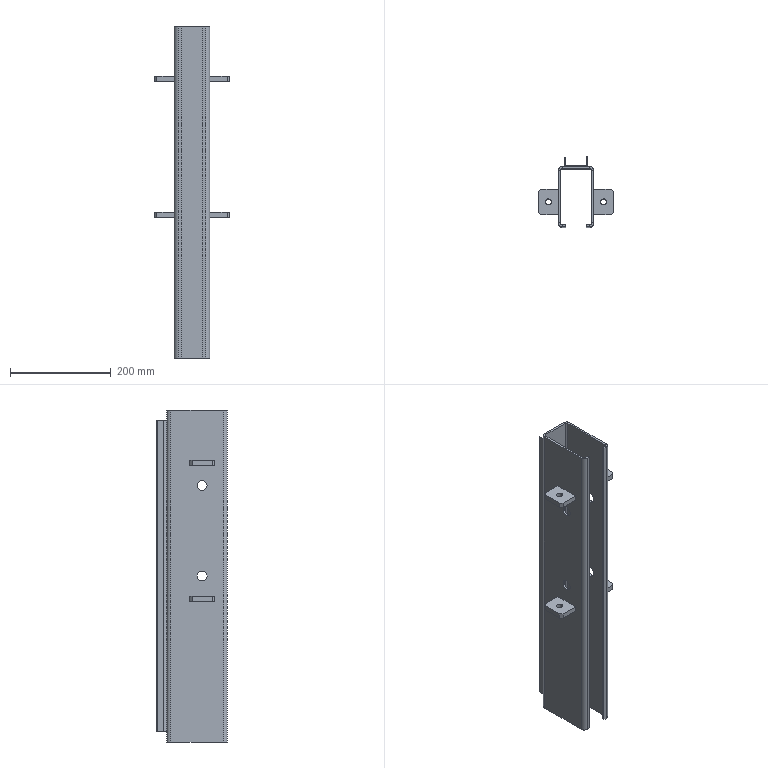Part | STEP file | 2 solids | 104 faces | box 150 x 140.041 x 660 mm | volume 992784 mm3 | plane 76 | cylinder 28 | commonest cylinder face diameters 12 x10 20 x8 8 x6 16 x4